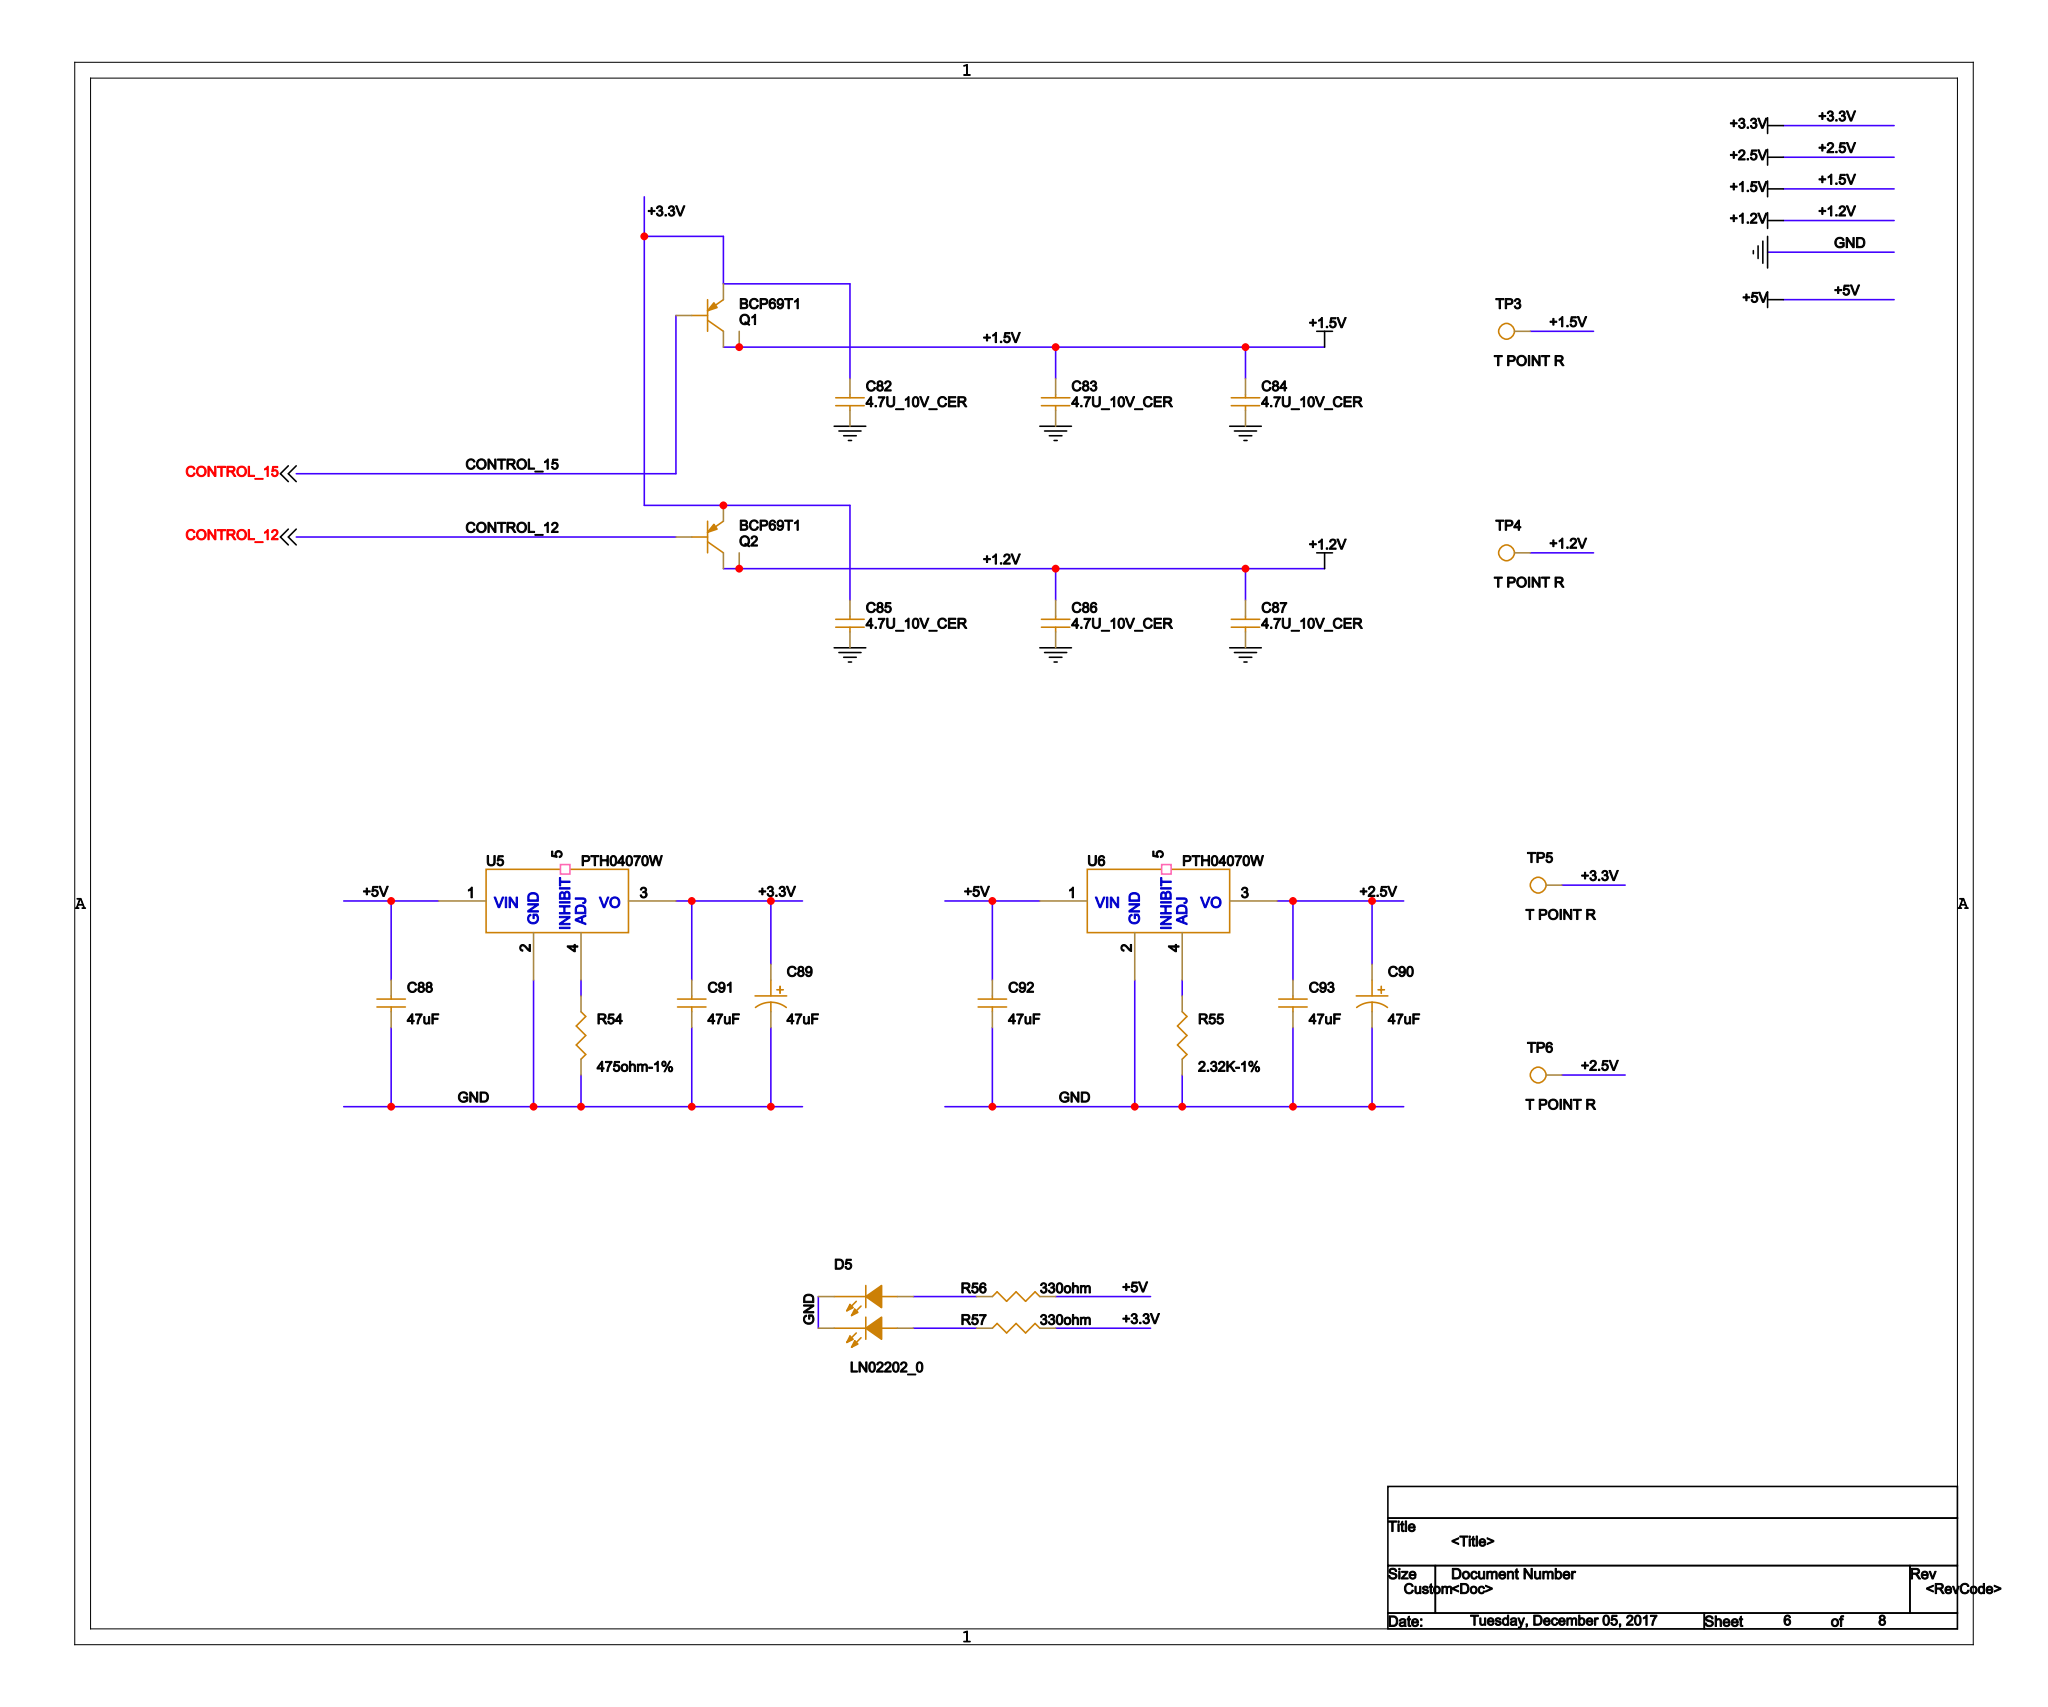Circuit board | Cadence Allegro | 219 parts | 174 nets | one sheet of the schematic
Parts on this sheet (reference | value | footprint):
C82 | 4.7U_10V_CER | SC0603
C83 | 4.7U_10V_CER | SC0603
C84 | 4.7U_10V_CER | SC0603
C85 | 4.7U_10V_CER | SC0603
C86 | 4.7U_10V_CER | SC0603
C87 | 4.7U_10V_CER | SC0603
C88 | 47uF | SC1210
C89 | 47uF | STC3528
C90 | 47uF | STC3528
C91 | 47uF | SC1210
C92 | 47uF | SC1210
C93 | 47uF | SC1210
D5 | LN02202_0 | LED_2
Q1 | BCP69T1 | SOT223
Q2 | BCP69T1 | SOT223
R54 | 475ohm-1% | SR0603
R55 | 2.32K-1% | SR0603
R56 | 330ohm | SR0603
R57 | 330ohm | SR0603
U5 | PTH04070W | PTH04070W
U6 | PTH04070W | PTH04070W
Nets of these parts (net: part-pin ...):
GND: C82-2 C83-2 C84-2 C85-2 C86-2 C87-2 C88-2 C89-2 C90-2 C91-2 C92-2 C93-2 D5-2 D5-4 R54-2 R55-2 U5-2 U6-2
CONTROL_12: Q2-1
CONTROL_15: Q1-1
+2.5V: C90-1 C93-1 U6-3
+1.5V: C83-1 C84-1 Q1-2 Q1-4
+1.2V: C86-1 C87-1 Q2-2 Q2-4
+3.3V: C82-1 C85-1 C89-1 C91-1 Q1-3 Q2-3 R57-2 U5-3
+5V: C88-1 C92-1 R56-2 U5-1 U6-1
N1398311: D5-1 R57-1
N1398289: D5-3 R56-1
N1334865: R54-1 U5-4
N1334572: R55-1 U6-4